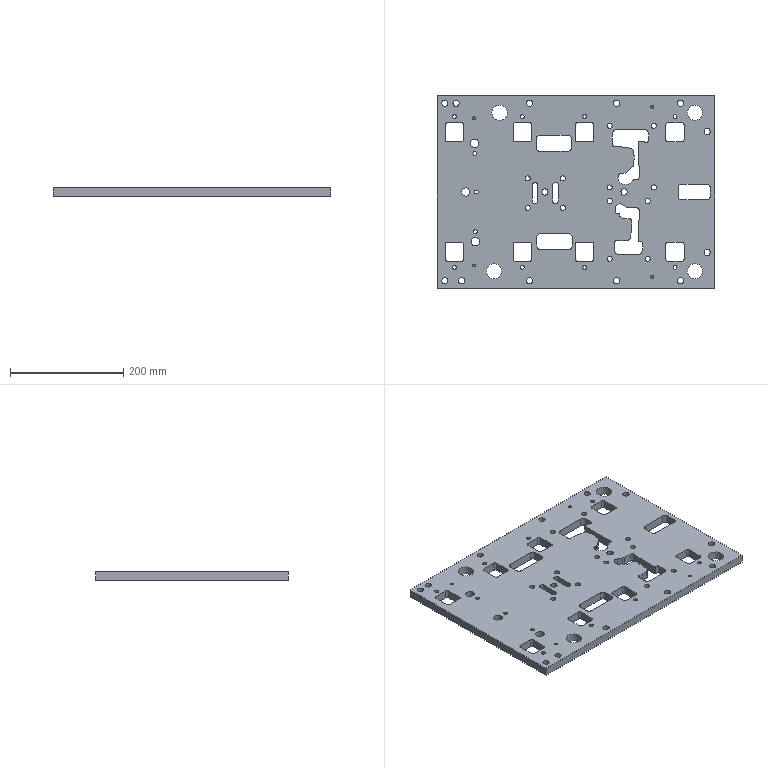Part | NX | features LIN_SOLID_COLOR 2 | 1 solid | 229 faces | box 490 x 340 x 15 mm | volume 2122302 mm3 | cylinder 125 | plane 96 | cone 4 | spline 4 | commonest cylinder face diameters 7 x32 11 x14 10 x13 9 x12 13 x12 6.8 x11